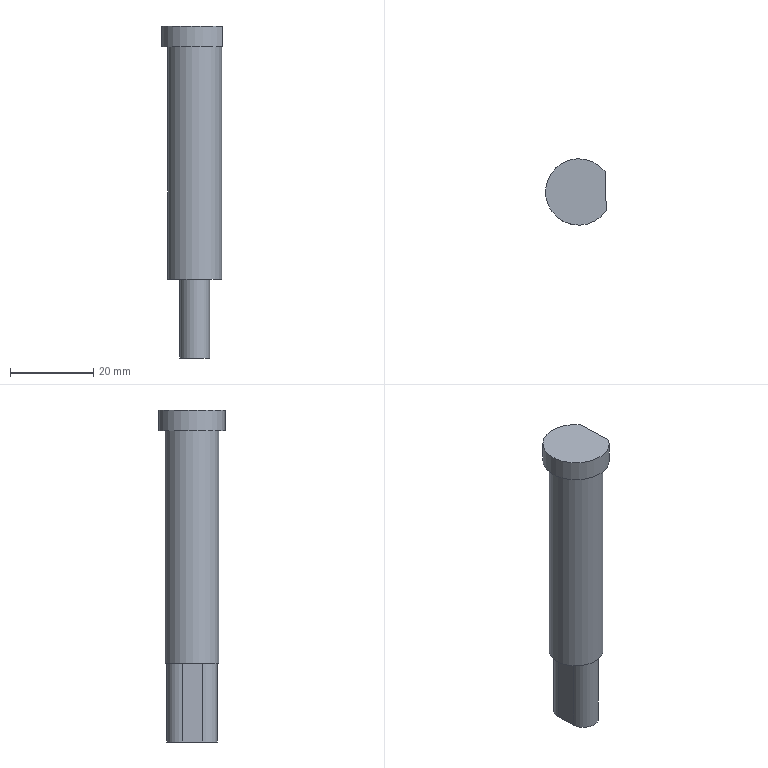Part | NX | features solid 2 | 1 solid | 11 faces | box 14.639 x 16 x 80 mm | volume 9817 mm3 | plane 7 | cylinder 4 | commonest cylinder face diameters 7.1 x2 13 x1 16 x1
STEP:
#1=CARTESIAN_POINT('',(145.222,252.444,32.));
#2=VERTEX_POINT('',#1);
#3=CARTESIAN_POINT('',(151.719,252.642,32.));
#4=DIRECTION('',(0.,0.,1.));
#5=DIRECTION('',(-0.9995,-0.03047,0.));
#6=AXIS2_PLACEMENT_3D('',#3,#4,#5);
#7=CIRCLE('',#6,6.5);
#8=EDGE_CURVE('',#2,#2,#7,.T.);
#9=ORIENTED_EDGE('',*,*,#8,.F.);
#10=EDGE_LOOP('',(#9));
#11=FACE_BOUND('',#10,.T.);
#12=CARTESIAN_POINT('',(148.247,250.035,32.));
#13=VERTEX_POINT('',#12);
#14=CARTESIAN_POINT('',(148.095,255.032,32.));
#15=VERTEX_POINT('',#14);
#16=CARTESIAN_POINT('',(148.171,252.534,32.));
#17=DIRECTION('',(-0.03047,0.9995,0.));
#18=VECTOR('',#17,1000.);
#19=LINE('',#16,#18);
#20=EDGE_CURVE('',#13,#15,#19,.T.);
#21=ORIENTED_EDGE('',*,*,#20,.F.);
#22=CARTESIAN_POINT('',(155.344,250.251,32.));
#23=VERTEX_POINT('',#22);
#24=CARTESIAN_POINT('',(151.795,250.143,32.));
#25=DIRECTION('',(0.,0.,1.));
#26=DIRECTION('',(-0.9995,-0.03047,0.));
#27=AXIS2_PLACEMENT_3D('',#24,#25,#26);
#28=CIRCLE('',#27,3.55);
#29=EDGE_CURVE('',#13,#23,#28,.T.);
#30=ORIENTED_EDGE('',*,*,#29,.T.);
#31=CARTESIAN_POINT('',(155.191,255.249,32.));
#32=VERTEX_POINT('',#31);
#33=CARTESIAN_POINT('',(155.268,252.75,32.));
#34=DIRECTION('',(-0.03047,0.9995,0.));
#35=VECTOR('',#34,1000.);
#36=LINE('',#33,#35);
#37=EDGE_CURVE('',#23,#32,#36,.T.);
#38=ORIENTED_EDGE('',*,*,#37,.T.);
#39=CARTESIAN_POINT('',(151.643,255.141,32.));
#40=DIRECTION('',(0.,0.,1.));
#41=DIRECTION('',(-0.9995,-0.03047,0.));
#42=AXIS2_PLACEMENT_3D('',#39,#40,#41);
#43=CIRCLE('',#42,3.55);
#44=EDGE_CURVE('',#32,#15,#43,.T.);
#45=ORIENTED_EDGE('',*,*,#44,.T.);
#46=EDGE_LOOP('',(#21,#30,#38,#45));
#47=FACE_BOUND('',#46,.T.);
#48=CARTESIAN_POINT('',(151.719,252.642,32.));
#49=DIRECTION('',(0.,0.,1.));
#50=DIRECTION('',(-0.9995,-0.03047,0.));
#51=AXIS2_PLACEMENT_3D('',#48,#49,#50);
#52=PLANE('',#51);
#53=ADVANCED_FACE('',(#11,#47),#52,.F.);
#54=ORIENTED_EDGE('',*,*,#8,.T.);
#55=EDGE_LOOP('',(#54));
#56=FACE_BOUND('',#55,.T.);
#57=CARTESIAN_POINT('',(158.216,252.84,88.));
#58=VERTEX_POINT('',#57);
#59=CARTESIAN_POINT('',(151.719,252.642,88.));
#60=DIRECTION('',(0.,0.,1.));
#61=DIRECTION('',(-0.9995,-0.03047,0.));
#62=AXIS2_PLACEMENT_3D('',#59,#60,#61);
#63=CIRCLE('',#62,6.5);
#64=EDGE_CURVE('',#58,#58,#63,.T.);
#65=ORIENTED_EDGE('',*,*,#64,.F.);
#66=EDGE_LOOP('',(#65));
#67=FACE_BOUND('',#66,.T.);
#68=CARTESIAN_POINT('',(151.719,252.642,93.));
#69=DIRECTION('',(0.,0.,-1.));
#70=DIRECTION('',(0.9995,0.03047,0.));
#71=AXIS2_PLACEMENT_3D('',#68,#69,#70);
#72=CYLINDRICAL_SURFACE('',#71,6.5);
#73=ADVANCED_FACE('',(#56,#67),#72,.T.);
#74=CARTESIAN_POINT('',(158.074,257.501,88.));
#75=VERTEX_POINT('',#74);
#76=CARTESIAN_POINT('',(158.358,248.178,88.));
#77=VERTEX_POINT('',#76);
#78=CARTESIAN_POINT('',(151.719,252.642,88.));
#79=DIRECTION('',(0.,0.,1.));
#80=DIRECTION('',(-0.9995,-0.03047,0.));
#81=AXIS2_PLACEMENT_3D('',#78,#79,#80);
#82=CIRCLE('',#81,8.);
#83=EDGE_CURVE('',#75,#77,#82,.T.);
#84=ORIENTED_EDGE('',*,*,#83,.F.);
#85=CARTESIAN_POINT('',(158.216,252.84,88.));
#86=DIRECTION('',(0.03047,-0.9995,0.));
#87=VECTOR('',#86,1000.);
#88=LINE('',#85,#87);
#89=EDGE_CURVE('',#75,#58,#88,.T.);
#90=ORIENTED_EDGE('',*,*,#89,.T.);
#91=ORIENTED_EDGE('',*,*,#64,.T.);
#92=CARTESIAN_POINT('',(158.216,252.84,88.));
#93=DIRECTION('',(0.03047,-0.9995,0.));
#94=VECTOR('',#93,1000.);
#95=LINE('',#92,#94);
#96=EDGE_CURVE('',#58,#77,#95,.T.);
#97=ORIENTED_EDGE('',*,*,#96,.T.);
#98=EDGE_LOOP('',(#84,#90,#91,#97));
#99=FACE_BOUND('',#98,.T.);
#100=CARTESIAN_POINT('',(151.719,252.642,88.));
#101=DIRECTION('',(0.,0.,1.));
#102=DIRECTION('',(-0.9995,-0.03047,0.));
#103=AXIS2_PLACEMENT_3D('',#100,#101,#102);
#104=PLANE('',#103);
#105=ADVANCED_FACE('',(#99),#104,.F.);
#106=CARTESIAN_POINT('',(158.358,248.178,93.));
#107=VERTEX_POINT('',#106);
#108=CARTESIAN_POINT('',(158.358,248.178,97.));
#109=DIRECTION('',(0.,0.,-1.));
#110=VECTOR('',#109,1000.);
#111=LINE('',#108,#110);
#112=EDGE_CURVE('',#77,#107,#111,.F.);
#113=ORIENTED_EDGE('',*,*,#112,.T.);
#114=CARTESIAN_POINT('',(158.074,257.501,93.));
#115=VERTEX_POINT('',#114);
#116=CARTESIAN_POINT('',(151.719,252.642,93.));
#117=DIRECTION('',(0.,0.,1.));
#118=DIRECTION('',(-0.9995,-0.03047,0.));
#119=AXIS2_PLACEMENT_3D('',#116,#117,#118);
#120=CIRCLE('',#119,8.);
#121=EDGE_CURVE('',#115,#107,#120,.T.);
#122=ORIENTED_EDGE('',*,*,#121,.F.);
#123=CARTESIAN_POINT('',(158.074,257.501,97.));
#124=DIRECTION('',(0.,0.,-1.));
#125=VECTOR('',#124,1000.);
#126=LINE('',#123,#125);
#127=EDGE_CURVE('',#115,#75,#126,.T.);
#128=ORIENTED_EDGE('',*,*,#127,.T.);
#129=ORIENTED_EDGE('',*,*,#83,.T.);
#130=EDGE_LOOP('',(#113,#122,#128,#129));
#131=FACE_BOUND('',#130,.T.);
#132=CARTESIAN_POINT('',(151.719,252.642,88.));
#133=DIRECTION('',(0.,0.,1.));
#134=DIRECTION('',(-0.9995,-0.03047,0.));
#135=AXIS2_PLACEMENT_3D('',#132,#133,#134);
#136=CYLINDRICAL_SURFACE('',#135,8.);
#137=ADVANCED_FACE('',(#131),#136,.T.);
#138=CARTESIAN_POINT('',(158.216,252.84,93.));
#139=DIRECTION('',(0.03047,-0.9995,0.));
#140=VECTOR('',#139,1000.);
#141=LINE('',#138,#140);
#142=EDGE_CURVE('',#115,#107,#141,.T.);
#143=ORIENTED_EDGE('',*,*,#142,.F.);
#144=ORIENTED_EDGE('',*,*,#121,.T.);
#145=EDGE_LOOP('',(#143,#144));
#146=FACE_BOUND('',#145,.T.);
#147=CARTESIAN_POINT('',(151.719,252.642,93.));
#148=DIRECTION('',(0.,0.,1.));
#149=DIRECTION('',(-0.9995,-0.03047,0.));
#150=AXIS2_PLACEMENT_3D('',#147,#148,#149);
#151=PLANE('',#150);
#152=ADVANCED_FACE('',(#146),#151,.T.);
#153=ORIENTED_EDGE('',*,*,#127,.F.);
#154=ORIENTED_EDGE('',*,*,#142,.T.);
#155=ORIENTED_EDGE('',*,*,#112,.F.);
#156=ORIENTED_EDGE('',*,*,#96,.F.);
#157=ORIENTED_EDGE('',*,*,#89,.F.);
#158=EDGE_LOOP('',(#153,#154,#155,#156,#157));
#159=FACE_BOUND('',#158,.T.);
#160=CARTESIAN_POINT('',(158.358,248.178,97.));
#161=DIRECTION('',(-0.9995,-0.03047,0.));
#162=DIRECTION('',(0.,0.,-1.));
#163=AXIS2_PLACEMENT_3D('',#160,#161,#162);
#164=PLANE('',#163);
#165=ADVANCED_FACE('',(#159),#164,.F.);
#166=CARTESIAN_POINT('',(148.247,250.035,13.));
#167=VERTEX_POINT('',#166);
#168=CARTESIAN_POINT('',(148.247,250.035,13.));
#169=DIRECTION('',(0.,0.,1.));
#170=VECTOR('',#169,1000.);
#171=LINE('',#168,#170);
#172=EDGE_CURVE('',#167,#13,#171,.T.);
#173=ORIENTED_EDGE('',*,*,#172,.T.);
#174=ORIENTED_EDGE('',*,*,#20,.T.);
#175=CARTESIAN_POINT('',(148.095,255.032,13.));
#176=VERTEX_POINT('',#175);
#177=CARTESIAN_POINT('',(148.095,255.032,13.));
#178=DIRECTION('',(0.,0.,1.));
#179=VECTOR('',#178,1000.);
#180=LINE('',#177,#179);
#181=EDGE_CURVE('',#176,#15,#180,.T.);
#182=ORIENTED_EDGE('',*,*,#181,.F.);
#183=CARTESIAN_POINT('',(148.247,250.035,13.));
#184=DIRECTION('',(-0.03047,0.9995,0.));
#185=VECTOR('',#184,1000.);
#186=LINE('',#183,#185);
#187=EDGE_CURVE('',#167,#176,#186,.T.);
#188=ORIENTED_EDGE('',*,*,#187,.F.);
#189=EDGE_LOOP('',(#173,#174,#182,#188));
#190=FACE_BOUND('',#189,.T.);
#191=CARTESIAN_POINT('',(148.247,250.035,13.));
#192=DIRECTION('',(0.9995,0.03047,0.));
#193=DIRECTION('',(0.,0.,1.));
#194=AXIS2_PLACEMENT_3D('',#191,#192,#193);
#195=PLANE('',#194);
#196=ADVANCED_FACE('',(#190),#195,.F.);
#197=ORIENTED_EDGE('',*,*,#44,.F.);
#198=CARTESIAN_POINT('',(155.191,255.249,13.));
#199=VERTEX_POINT('',#198);
#200=CARTESIAN_POINT('',(155.191,255.249,13.));
#201=DIRECTION('',(0.,0.,1.));
#202=VECTOR('',#201,1000.);
#203=LINE('',#200,#202);
#204=EDGE_CURVE('',#199,#32,#203,.T.);
#205=ORIENTED_EDGE('',*,*,#204,.F.);
#206=CARTESIAN_POINT('',(151.643,255.141,13.));
#207=DIRECTION('',(0.,0.,1.));
#208=DIRECTION('',(-0.9995,-0.03047,0.));
#209=AXIS2_PLACEMENT_3D('',#206,#207,#208);
#210=CIRCLE('',#209,3.55);
#211=EDGE_CURVE('',#199,#176,#210,.T.);
#212=ORIENTED_EDGE('',*,*,#211,.T.);
#213=ORIENTED_EDGE('',*,*,#181,.T.);
#214=EDGE_LOOP('',(#197,#205,#212,#213));
#215=FACE_BOUND('',#214,.T.);
#216=CARTESIAN_POINT('',(151.643,255.141,13.));
#217=DIRECTION('',(0.,0.,1.));
#218=DIRECTION('',(-0.9995,-0.03047,0.));
#219=AXIS2_PLACEMENT_3D('',#216,#217,#218);
#220=CYLINDRICAL_SURFACE('',#219,3.55);
#221=ADVANCED_FACE('',(#215),#220,.T.);
#222=ORIENTED_EDGE('',*,*,#37,.F.);
#223=CARTESIAN_POINT('',(155.344,250.251,13.));
#224=VERTEX_POINT('',#223);
#225=CARTESIAN_POINT('',(155.344,250.251,13.));
#226=DIRECTION('',(0.,0.,1.));
#227=VECTOR('',#226,1000.);
#228=LINE('',#225,#227);
#229=EDGE_CURVE('',#224,#23,#228,.T.);
#230=ORIENTED_EDGE('',*,*,#229,.F.);
#231=CARTESIAN_POINT('',(155.344,250.251,13.));
#232=DIRECTION('',(-0.03047,0.9995,0.));
#233=VECTOR('',#232,1000.);
#234=LINE('',#231,#233);
#235=EDGE_CURVE('',#224,#199,#234,.T.);
#236=ORIENTED_EDGE('',*,*,#235,.T.);
#237=ORIENTED_EDGE('',*,*,#204,.T.);
#238=EDGE_LOOP('',(#222,#230,#236,#237));
#239=FACE_BOUND('',#238,.T.);
#240=CARTESIAN_POINT('',(155.344,250.251,13.));
#241=DIRECTION('',(0.9995,0.03047,0.));
#242=DIRECTION('',(0.,0.,1.));
#243=AXIS2_PLACEMENT_3D('',#240,#241,#242);
#244=PLANE('',#243);
#245=ADVANCED_FACE('',(#239),#244,.T.);
#246=ORIENTED_EDGE('',*,*,#29,.F.);
#247=ORIENTED_EDGE('',*,*,#172,.F.);
#248=CARTESIAN_POINT('',(151.795,250.143,13.));
#249=DIRECTION('',(0.,0.,1.));
#250=DIRECTION('',(-0.9995,-0.03047,0.));
#251=AXIS2_PLACEMENT_3D('',#248,#249,#250);
#252=CIRCLE('',#251,3.55);
#253=EDGE_CURVE('',#167,#224,#252,.T.);
#254=ORIENTED_EDGE('',*,*,#253,.T.);
#255=ORIENTED_EDGE('',*,*,#229,.T.);
#256=EDGE_LOOP('',(#246,#247,#254,#255));
#257=FACE_BOUND('',#256,.T.);
#258=CARTESIAN_POINT('',(151.795,250.143,13.));
#259=DIRECTION('',(0.,0.,1.));
#260=DIRECTION('',(-0.9995,-0.03047,0.));
#261=AXIS2_PLACEMENT_3D('',#258,#259,#260);
#262=CYLINDRICAL_SURFACE('',#261,3.55);
#263=ADVANCED_FACE('',(#257),#262,.T.);
#264=ORIENTED_EDGE('',*,*,#187,.T.);
#265=ORIENTED_EDGE('',*,*,#211,.F.);
#266=ORIENTED_EDGE('',*,*,#235,.F.);
#267=ORIENTED_EDGE('',*,*,#253,.F.);
#268=EDGE_LOOP('',(#264,#265,#266,#267));
#269=FACE_BOUND('',#268,.T.);
#270=CARTESIAN_POINT('',(151.643,255.141,13.));
#271=DIRECTION('',(0.,0.,1.));
#272=DIRECTION('',(-0.9995,-0.03047,0.));
#273=AXIS2_PLACEMENT_3D('',#270,#271,#272);
#274=PLANE('',#273);
#275=ADVANCED_FACE('',(#269),#274,.F.);
#276=CLOSED_SHELL('',(#53,#73,#105,#137,#152,#165,#196,#221,#245,#263,#275));
#277=MANIFOLD_SOLID_BREP('',#276);
#278=(LENGTH_UNIT()NAMED_UNIT(*)SI_UNIT(.MILLI.,.METRE.));
#279=UNCERTAINTY_MEASURE_WITH_UNIT(LENGTH_MEASURE(0.00001),#278,'','');
#280=(NAMED_UNIT(*)PLANE_ANGLE_UNIT()SI_UNIT($,.RADIAN.));
#281=(NAMED_UNIT(*)SI_UNIT($,.STERADIAN.)SOLID_ANGLE_UNIT());
#282=(GEOMETRIC_REPRESENTATION_CONTEXT(3)GLOBAL_UNCERTAINTY_ASSIGNED_CONTEXT((#279))GLOBAL_UNIT_ASSIGNED_CONTEXT((#278,#280,#281))REPRESENTATION_CONTEXT('',''));
#283=ADVANCED_BREP_SHAPE_REPRESENTATION('',(#277),#282);